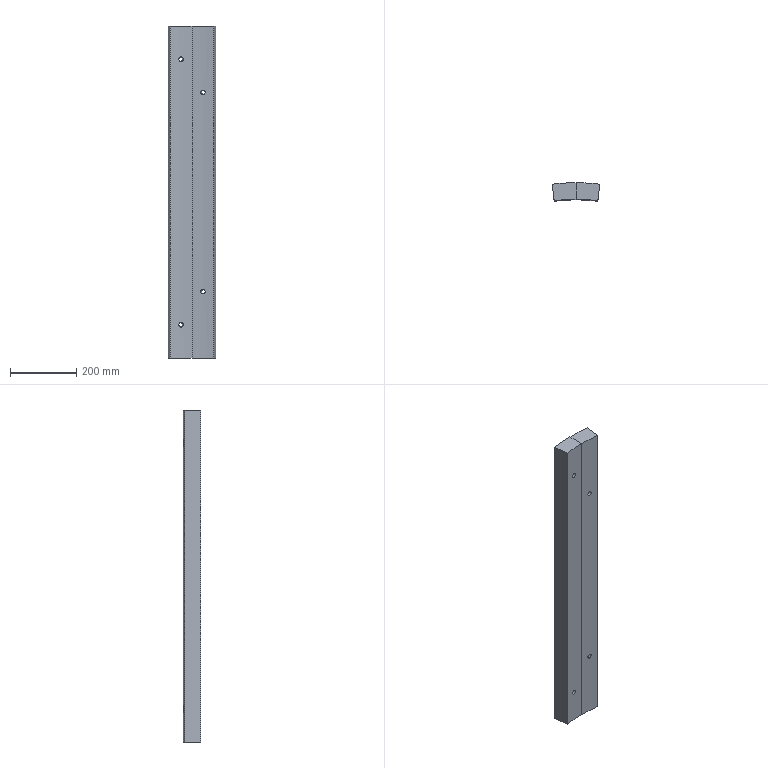Part | SolidWorks | features 3DProfileFeature 2, HoleWzd 2, MirrorPattern 2, Extrusion 1, ICE 1 | 2 solids | 32 faces | box 143.632 x 54.124 x 1000 mm | volume 6848220 mm3 | cylinder 20 | plane 12 | commonest cylinder face diameters 13.5 x8 23.78 x8 1046 x2 1146 x2